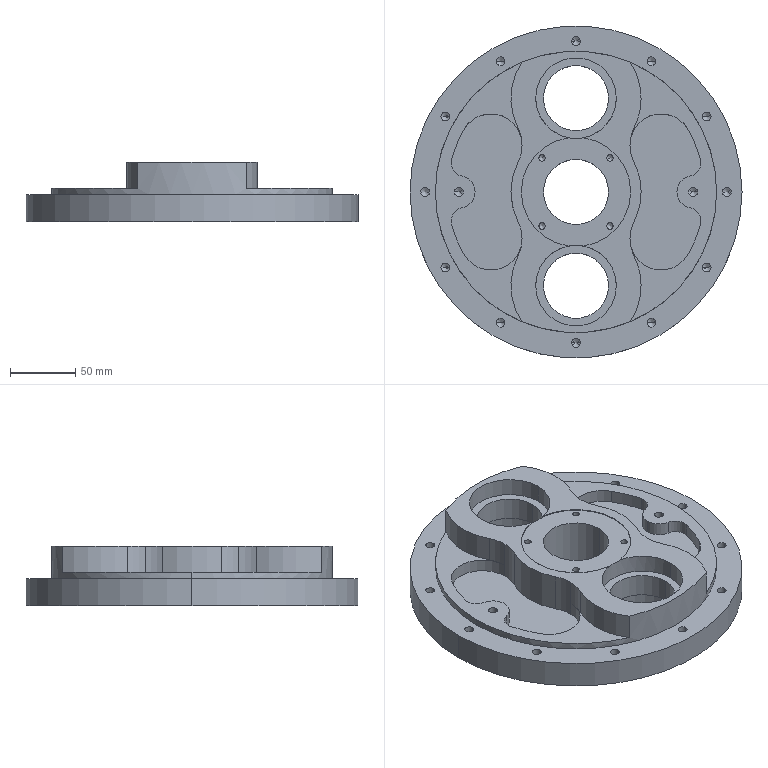Part | STEP file | Guide disc SGN-2-04 | 1 solid | 153 faces | box 255 x 255 x 46 mm | volume 1203695 mm3 | cylinder 97 | cone 44 | plane 12 | commonest cylinder face diameters 6.8 x36 100 x9 5 x8 62 x8 20 x6 50 x6